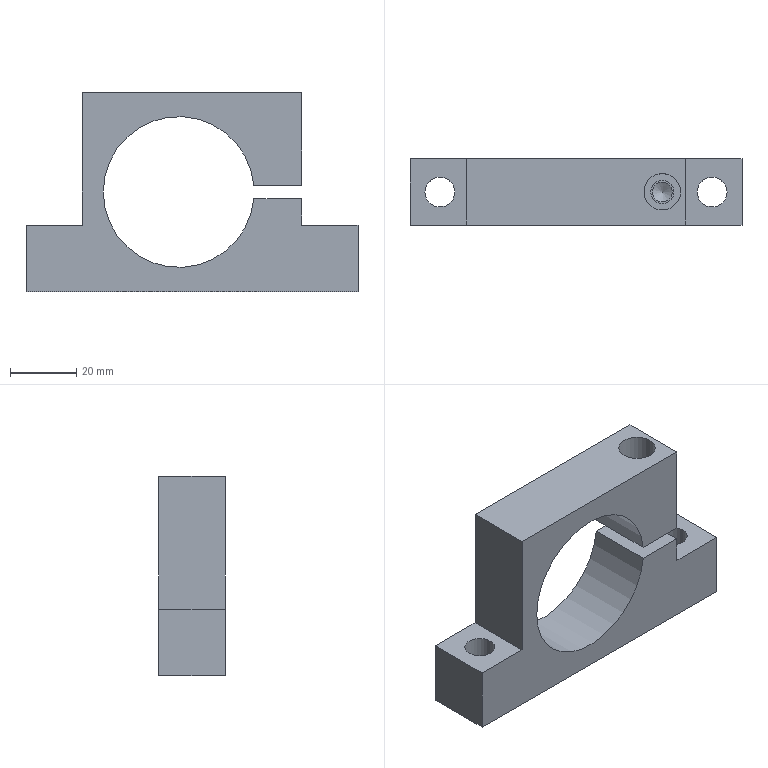Part | NX | features MAIN_BODY 2 | 1 solid | 21 faces | box 100 x 20 x 60 mm | volume 53801 mm3 | plane 14 | cylinder 6 | cone 1 | commonest cylinder face diameters 9 x2 6 x1 7 x1 11 x1 45.4 x1
STEP:
#1=CARTESIAN_POINT('',(568.,600.,-213.));
#2=VERTEX_POINT('',#1);
#3=CARTESIAN_POINT('',(568.,600.,-185.));
#4=VERTEX_POINT('',#3);
#5=CARTESIAN_POINT('',(568.,600.,-185.));
#6=DIRECTION('',(0.,0.,1.));
#7=VECTOR('',#6,1000.);
#8=LINE('',#5,#7);
#9=EDGE_CURVE('',#2,#4,#8,.T.);
#10=ORIENTED_EDGE('',*,*,#9,.F.);
#11=CARTESIAN_POINT('',(568.,620.,-213.));
#12=VERTEX_POINT('',#11);
#13=CARTESIAN_POINT('',(568.,600.,-213.));
#14=DIRECTION('',(0.,-1.,0.));
#15=VECTOR('',#14,1000.);
#16=LINE('',#13,#15);
#17=EDGE_CURVE('',#12,#2,#16,.T.);
#18=ORIENTED_EDGE('',*,*,#17,.F.);
#19=CARTESIAN_POINT('',(568.,620.,-185.));
#20=VERTEX_POINT('',#19);
#21=CARTESIAN_POINT('',(568.,620.,-185.));
#22=DIRECTION('',(0.,0.,1.));
#23=VECTOR('',#22,1000.);
#24=LINE('',#21,#23);
#25=EDGE_CURVE('',#12,#20,#24,.T.);
#26=ORIENTED_EDGE('',*,*,#25,.T.);
#27=CARTESIAN_POINT('',(568.,565.,-185.));
#28=DIRECTION('',(0.,1.,0.));
#29=VECTOR('',#28,1000.);
#30=LINE('',#27,#29);
#31=EDGE_CURVE('',#4,#20,#30,.T.);
#32=ORIENTED_EDGE('',*,*,#31,.F.);
#33=EDGE_LOOP('',(#10,#18,#26,#32));
#34=FACE_BOUND('',#33,.T.);
#35=CARTESIAN_POINT('',(568.,565.,-225.));
#36=DIRECTION('',(-1.,0.,0.));
#37=DIRECTION('',(0.,0.,-1.));
#38=AXIS2_PLACEMENT_3D('',#35,#36,#37);
#39=PLANE('',#38);
#40=ADVANCED_FACE('',(#34),#39,.F.);
#41=CARTESIAN_POINT('',(485.,600.,-225.));
#42=VERTEX_POINT('',#41);
#43=CARTESIAN_POINT('',(485.,620.,-225.));
#44=VERTEX_POINT('',#43);
#45=CARTESIAN_POINT('',(485.,565.,-225.));
#46=DIRECTION('',(0.,1.,0.));
#47=VECTOR('',#46,1000.);
#48=LINE('',#45,#47);
#49=EDGE_CURVE('',#42,#44,#48,.T.);
#50=ORIENTED_EDGE('',*,*,#49,.T.);
#51=CARTESIAN_POINT('',(485.,620.,-245.));
#52=VERTEX_POINT('',#51);
#53=CARTESIAN_POINT('',(485.,620.,-245.));
#54=DIRECTION('',(0.,0.,1.));
#55=VECTOR('',#54,1000.);
#56=LINE('',#53,#55);
#57=EDGE_CURVE('',#52,#44,#56,.T.);
#58=ORIENTED_EDGE('',*,*,#57,.F.);
#59=CARTESIAN_POINT('',(485.,600.,-245.));
#60=VERTEX_POINT('',#59);
#61=CARTESIAN_POINT('',(485.,600.,-245.));
#62=DIRECTION('',(0.,1.,0.));
#63=VECTOR('',#62,1000.);
#64=LINE('',#61,#63);
#65=EDGE_CURVE('',#60,#52,#64,.T.);
#66=ORIENTED_EDGE('',*,*,#65,.F.);
#67=CARTESIAN_POINT('',(485.,600.,-245.));
#68=DIRECTION('',(0.,0.,1.));
#69=VECTOR('',#68,1000.);
#70=LINE('',#67,#69);
#71=EDGE_CURVE('',#60,#42,#70,.T.);
#72=ORIENTED_EDGE('',*,*,#71,.T.);
#73=EDGE_LOOP('',(#50,#58,#66,#72));
#74=FACE_BOUND('',#73,.T.);
#75=CARTESIAN_POINT('',(485.,600.,-245.));
#76=DIRECTION('',(-1.,0.,0.));
#77=DIRECTION('',(0.,0.,-1.));
#78=AXIS2_PLACEMENT_3D('',#75,#76,#77);
#79=PLANE('',#78);
#80=ADVANCED_FACE('',(#74),#79,.T.);
#81=CARTESIAN_POINT('',(555.5,610.,-185.));
#82=VERTEX_POINT('',#81);
#83=CARTESIAN_POINT('',(561.,610.,-185.));
#84=DIRECTION('',(0.,0.,-1.));
#85=DIRECTION('',(-1.,0.,0.));
#86=AXIS2_PLACEMENT_3D('',#83,#84,#85);
#87=CIRCLE('',#86,5.5);
#88=EDGE_CURVE('',#82,#82,#87,.T.);
#89=ORIENTED_EDGE('',*,*,#88,.T.);
#90=EDGE_LOOP('',(#89));
#91=FACE_BOUND('',#90,.T.);
#92=ORIENTED_EDGE('',*,*,#31,.T.);
#93=CARTESIAN_POINT('',(502.,620.,-185.));
#94=VERTEX_POINT('',#93);
#95=CARTESIAN_POINT('',(485.,620.,-185.));
#96=DIRECTION('',(1.,0.,0.));
#97=VECTOR('',#96,1000.);
#98=LINE('',#95,#97);
#99=EDGE_CURVE('',#94,#20,#98,.T.);
#100=ORIENTED_EDGE('',*,*,#99,.F.);
#101=CARTESIAN_POINT('',(502.,600.,-185.));
#102=VERTEX_POINT('',#101);
#103=CARTESIAN_POINT('',(502.,565.,-185.));
#104=DIRECTION('',(0.,1.,0.));
#105=VECTOR('',#104,1000.);
#106=LINE('',#103,#105);
#107=EDGE_CURVE('',#102,#94,#106,.T.);
#108=ORIENTED_EDGE('',*,*,#107,.F.);
#109=CARTESIAN_POINT('',(485.,600.,-185.));
#110=DIRECTION('',(1.,0.,0.));
#111=VECTOR('',#110,1000.);
#112=LINE('',#109,#111);
#113=EDGE_CURVE('',#102,#4,#112,.T.);
#114=ORIENTED_EDGE('',*,*,#113,.T.);
#115=EDGE_LOOP('',(#92,#100,#108,#114));
#116=FACE_BOUND('',#115,.T.);
#117=CARTESIAN_POINT('',(485.,600.,-185.));
#118=DIRECTION('',(0.,0.,1.));
#119=DIRECTION('',(0.,-1.,0.));
#120=AXIS2_PLACEMENT_3D('',#117,#118,#119);
#121=PLANE('',#120);
#122=ADVANCED_FACE('',(#91,#116),#121,.T.);
#123=CARTESIAN_POINT('',(585.,600.,-225.));
#124=VERTEX_POINT('',#123);
#125=CARTESIAN_POINT('',(585.,620.,-225.));
#126=VERTEX_POINT('',#125);
#127=CARTESIAN_POINT('',(585.,565.,-225.));
#128=DIRECTION('',(0.,1.,0.));
#129=VECTOR('',#128,1000.);
#130=LINE('',#127,#129);
#131=EDGE_CURVE('',#124,#126,#130,.T.);
#132=ORIENTED_EDGE('',*,*,#131,.F.);
#133=CARTESIAN_POINT('',(585.,600.,-245.));
#134=VERTEX_POINT('',#133);
#135=CARTESIAN_POINT('',(585.,600.,-185.));
#136=DIRECTION('',(0.,0.,-1.));
#137=VECTOR('',#136,1000.);
#138=LINE('',#135,#137);
#139=EDGE_CURVE('',#124,#134,#138,.T.);
#140=ORIENTED_EDGE('',*,*,#139,.T.);
#141=CARTESIAN_POINT('',(585.,620.,-245.));
#142=VERTEX_POINT('',#141);
#143=CARTESIAN_POINT('',(585.,600.,-245.));
#144=DIRECTION('',(0.,1.,0.));
#145=VECTOR('',#144,1000.);
#146=LINE('',#143,#145);
#147=EDGE_CURVE('',#134,#142,#146,.T.);
#148=ORIENTED_EDGE('',*,*,#147,.T.);
#149=CARTESIAN_POINT('',(585.,620.,-185.));
#150=DIRECTION('',(0.,0.,-1.));
#151=VECTOR('',#150,1000.);
#152=LINE('',#149,#151);
#153=EDGE_CURVE('',#126,#142,#152,.T.);
#154=ORIENTED_EDGE('',*,*,#153,.F.);
#155=EDGE_LOOP('',(#132,#140,#148,#154));
#156=FACE_BOUND('',#155,.T.);
#157=CARTESIAN_POINT('',(585.,600.,-185.));
#158=DIRECTION('',(1.,0.,0.));
#159=DIRECTION('',(0.,0.,1.));
#160=AXIS2_PLACEMENT_3D('',#157,#158,#159);
#161=PLANE('',#160);
#162=ADVANCED_FACE('',(#156),#161,.T.);
#163=CARTESIAN_POINT('',(580.5,610.,-245.));
#164=VERTEX_POINT('',#163);
#165=CARTESIAN_POINT('',(576.,610.,-245.));
#166=DIRECTION('',(0.,0.,-1.));
#167=DIRECTION('',(1.,0.,0.));
#168=AXIS2_PLACEMENT_3D('',#165,#166,#167);
#169=CIRCLE('',#168,4.5);
#170=EDGE_CURVE('',#164,#164,#169,.T.);
#171=ORIENTED_EDGE('',*,*,#170,.F.);
#172=EDGE_LOOP('',(#171));
#173=FACE_BOUND('',#172,.T.);
#174=CARTESIAN_POINT('',(498.5,610.,-245.));
#175=VERTEX_POINT('',#174);
#176=CARTESIAN_POINT('',(494.,610.,-245.));
#177=DIRECTION('',(0.,0.,-1.));
#178=DIRECTION('',(1.,0.,0.));
#179=AXIS2_PLACEMENT_3D('',#176,#177,#178);
#180=CIRCLE('',#179,4.5);
#181=EDGE_CURVE('',#175,#175,#180,.T.);
#182=ORIENTED_EDGE('',*,*,#181,.F.);
#183=EDGE_LOOP('',(#182));
#184=FACE_BOUND('',#183,.T.);
#185=CARTESIAN_POINT('',(585.,620.,-245.));
#186=DIRECTION('',(-1.,0.,0.));
#187=VECTOR('',#186,1000.);
#188=LINE('',#185,#187);
#189=EDGE_CURVE('',#142,#52,#188,.T.);
#190=ORIENTED_EDGE('',*,*,#189,.F.);
#191=ORIENTED_EDGE('',*,*,#147,.F.);
#192=CARTESIAN_POINT('',(585.,600.,-245.));
#193=DIRECTION('',(-1.,0.,0.));
#194=VECTOR('',#193,1000.);
#195=LINE('',#192,#194);
#196=EDGE_CURVE('',#134,#60,#195,.T.);
#197=ORIENTED_EDGE('',*,*,#196,.T.);
#198=ORIENTED_EDGE('',*,*,#65,.T.);
#199=EDGE_LOOP('',(#190,#191,#197,#198));
#200=FACE_BOUND('',#199,.T.);
#201=CARTESIAN_POINT('',(585.,600.,-245.));
#202=DIRECTION('',(0.,0.,-1.));
#203=DIRECTION('',(1.,0.,0.));
#204=AXIS2_PLACEMENT_3D('',#201,#202,#203);
#205=PLANE('',#204);
#206=ADVANCED_FACE('',(#173,#184,#200),#205,.T.);
#207=CARTESIAN_POINT('',(553.612,600.,-213.));
#208=VERTEX_POINT('',#207);
#209=CARTESIAN_POINT('',(553.612,620.,-213.));
#210=VERTEX_POINT('',#209);
#211=CARTESIAN_POINT('',(553.612,600.,-213.));
#212=DIRECTION('',(0.,1.,0.));
#213=VECTOR('',#212,1000.);
#214=LINE('',#211,#213);
#215=EDGE_CURVE('',#208,#210,#214,.T.);
#216=ORIENTED_EDGE('',*,*,#215,.F.);
#217=CARTESIAN_POINT('',(553.612,600.,-217.));
#218=VERTEX_POINT('',#217);
#219=CARTESIAN_POINT('',(531.,600.,-215.));
#220=DIRECTION('',(0.,-1.,0.));
#221=DIRECTION('',(1.,0.,0.));
#222=AXIS2_PLACEMENT_3D('',#219,#220,#221);
#223=CIRCLE('',#222,22.7);
#224=EDGE_CURVE('',#208,#218,#223,.T.);
#225=ORIENTED_EDGE('',*,*,#224,.T.);
#226=CARTESIAN_POINT('',(553.612,620.,-217.));
#227=VERTEX_POINT('',#226);
#228=CARTESIAN_POINT('',(553.612,600.,-217.));
#229=DIRECTION('',(0.,1.,0.));
#230=VECTOR('',#229,1000.);
#231=LINE('',#228,#230);
#232=EDGE_CURVE('',#227,#218,#231,.F.);
#233=ORIENTED_EDGE('',*,*,#232,.F.);
#234=CARTESIAN_POINT('',(531.,620.,-215.));
#235=DIRECTION('',(0.,-1.,0.));
#236=DIRECTION('',(1.,0.,0.));
#237=AXIS2_PLACEMENT_3D('',#234,#235,#236);
#238=CIRCLE('',#237,22.7);
#239=EDGE_CURVE('',#210,#227,#238,.T.);
#240=ORIENTED_EDGE('',*,*,#239,.F.);
#241=EDGE_LOOP('',(#216,#225,#233,#240));
#242=FACE_BOUND('',#241,.T.);
#243=CARTESIAN_POINT('',(531.,600.,-215.));
#244=DIRECTION('',(0.,1.,0.));
#245=DIRECTION('',(-1.,0.,0.));
#246=AXIS2_PLACEMENT_3D('',#243,#244,#245);
#247=CYLINDRICAL_SURFACE('',#246,22.7);
#248=ADVANCED_FACE('',(#242),#247,.F.);
#249=ORIENTED_EDGE('',*,*,#224,.F.);
#250=CARTESIAN_POINT('',(531.,600.,-213.));
#251=DIRECTION('',(1.,0.,0.));
#252=VECTOR('',#251,1000.);
#253=LINE('',#250,#252);
#254=EDGE_CURVE('',#208,#2,#253,.T.);
#255=ORIENTED_EDGE('',*,*,#254,.T.);
#256=ORIENTED_EDGE('',*,*,#9,.T.);
#257=ORIENTED_EDGE('',*,*,#113,.F.);
#258=CARTESIAN_POINT('',(502.,600.,-225.));
#259=VERTEX_POINT('',#258);
#260=CARTESIAN_POINT('',(502.,600.,-185.));
#261=DIRECTION('',(0.,0.,-1.));
#262=VECTOR('',#261,1000.);
#263=LINE('',#260,#262);
#264=EDGE_CURVE('',#102,#259,#263,.T.);
#265=ORIENTED_EDGE('',*,*,#264,.T.);
#266=CARTESIAN_POINT('',(485.,600.,-225.));
#267=DIRECTION('',(-1.,0.,0.));
#268=VECTOR('',#267,1000.);
#269=LINE('',#266,#268);
#270=EDGE_CURVE('',#259,#42,#269,.T.);
#271=ORIENTED_EDGE('',*,*,#270,.T.);
#272=ORIENTED_EDGE('',*,*,#71,.F.);
#273=ORIENTED_EDGE('',*,*,#196,.F.);
#274=ORIENTED_EDGE('',*,*,#139,.F.);
#275=CARTESIAN_POINT('',(568.,600.,-225.));
#276=VERTEX_POINT('',#275);
#277=CARTESIAN_POINT('',(485.,600.,-225.));
#278=DIRECTION('',(-1.,0.,0.));
#279=VECTOR('',#278,1000.);
#280=LINE('',#277,#279);
#281=EDGE_CURVE('',#124,#276,#280,.T.);
#282=ORIENTED_EDGE('',*,*,#281,.T.);
#283=CARTESIAN_POINT('',(568.,600.,-217.));
#284=VERTEX_POINT('',#283);
#285=CARTESIAN_POINT('',(568.,600.,-185.));
#286=DIRECTION('',(0.,0.,1.));
#287=VECTOR('',#286,1000.);
#288=LINE('',#285,#287);
#289=EDGE_CURVE('',#276,#284,#288,.T.);
#290=ORIENTED_EDGE('',*,*,#289,.T.);
#291=CARTESIAN_POINT('',(531.,600.,-217.));
#292=DIRECTION('',(1.,0.,0.));
#293=VECTOR('',#292,1000.);
#294=LINE('',#291,#293);
#295=EDGE_CURVE('',#218,#284,#294,.T.);
#296=ORIENTED_EDGE('',*,*,#295,.F.);
#297=EDGE_LOOP('',(#249,#255,#256,#257,#265,#271,#272,#273,#274,#282,#290,#296));
#298=FACE_BOUND('',#297,.T.);
#299=CARTESIAN_POINT('',(485.,600.,-185.));
#300=DIRECTION('',(0.,1.,0.));
#301=DIRECTION('',(-1.,0.,0.));
#302=AXIS2_PLACEMENT_3D('',#299,#300,#301);
#303=PLANE('',#302);
#304=ADVANCED_FACE('',(#298),#303,.F.);
#305=CARTESIAN_POINT('',(485.,620.,-213.));
#306=DIRECTION('',(1.,0.,0.));
#307=VECTOR('',#306,1000.);
#308=LINE('',#305,#307);
#309=EDGE_CURVE('',#210,#12,#308,.T.);
#310=ORIENTED_EDGE('',*,*,#309,.F.);
#311=ORIENTED_EDGE('',*,*,#239,.T.);
#312=CARTESIAN_POINT('',(568.,620.,-217.));
#313=VERTEX_POINT('',#312);
#314=CARTESIAN_POINT('',(485.,620.,-217.));
#315=DIRECTION('',(1.,0.,0.));
#316=VECTOR('',#315,1000.);
#317=LINE('',#314,#316);
#318=EDGE_CURVE('',#313,#227,#317,.F.);
#319=ORIENTED_EDGE('',*,*,#318,.F.);
#320=CARTESIAN_POINT('',(568.,620.,-225.));
#321=VERTEX_POINT('',#320);
#322=CARTESIAN_POINT('',(568.,620.,-185.));
#323=DIRECTION('',(0.,0.,1.));
#324=VECTOR('',#323,1000.);
#325=LINE('',#322,#324);
#326=EDGE_CURVE('',#321,#313,#325,.T.);
#327=ORIENTED_EDGE('',*,*,#326,.F.);
#328=CARTESIAN_POINT('',(485.,620.,-225.));
#329=DIRECTION('',(-1.,0.,0.));
#330=VECTOR('',#329,1000.);
#331=LINE('',#328,#330);
#332=EDGE_CURVE('',#126,#321,#331,.T.);
#333=ORIENTED_EDGE('',*,*,#332,.F.);
#334=ORIENTED_EDGE('',*,*,#153,.T.);
#335=ORIENTED_EDGE('',*,*,#189,.T.);
#336=ORIENTED_EDGE('',*,*,#57,.T.);
#337=CARTESIAN_POINT('',(502.,620.,-225.));
#338=VERTEX_POINT('',#337);
#339=CARTESIAN_POINT('',(485.,620.,-225.));
#340=DIRECTION('',(-1.,0.,0.));
#341=VECTOR('',#340,1000.);
#342=LINE('',#339,#341);
#343=EDGE_CURVE('',#338,#44,#342,.T.);
#344=ORIENTED_EDGE('',*,*,#343,.F.);
#345=CARTESIAN_POINT('',(502.,620.,-185.));
#346=DIRECTION('',(0.,0.,-1.));
#347=VECTOR('',#346,1000.);
#348=LINE('',#345,#347);
#349=EDGE_CURVE('',#94,#338,#348,.T.);
#350=ORIENTED_EDGE('',*,*,#349,.F.);
#351=ORIENTED_EDGE('',*,*,#99,.T.);
#352=ORIENTED_EDGE('',*,*,#25,.F.);
#353=EDGE_LOOP('',(#310,#311,#319,#327,#333,#334,#335,#336,#344,#350,#351,#352));
#354=FACE_BOUND('',#353,.T.);
#355=CARTESIAN_POINT('',(485.,620.,-185.));
#356=DIRECTION('',(0.,1.,0.));
#357=DIRECTION('',(-1.,0.,0.));
#358=AXIS2_PLACEMENT_3D('',#355,#356,#357);
#359=PLANE('',#358);
#360=ADVANCED_FACE('',(#354),#359,.T.);
#361=ORIENTED_EDGE('',*,*,#107,.T.);
#362=ORIENTED_EDGE('',*,*,#349,.T.);
#363=CARTESIAN_POINT('',(502.,565.,-225.));
#364=DIRECTION('',(0.,1.,0.));
#365=VECTOR('',#364,1000.);
#366=LINE('',#363,#365);
#367=EDGE_CURVE('',#259,#338,#366,.T.);
#368=ORIENTED_EDGE('',*,*,#367,.F.);
#369=ORIENTED_EDGE('',*,*,#264,.F.);
#370=EDGE_LOOP('',(#361,#362,#368,#369));
#371=FACE_BOUND('',#370,.T.);
#372=CARTESIAN_POINT('',(502.,565.,-185.));
#373=DIRECTION('',(1.,0.,0.));
#374=DIRECTION('',(0.,0.,1.));
#375=AXIS2_PLACEMENT_3D('',#372,#373,#374);
#376=PLANE('',#375);
#377=ADVANCED_FACE('',(#371),#376,.F.);
#378=CARTESIAN_POINT('',(498.5,610.,-225.));
#379=VERTEX_POINT('',#378);
#380=CARTESIAN_POINT('',(494.,610.,-225.));
#381=DIRECTION('',(0.,0.,-1.));
#382=DIRECTION('',(1.,0.,0.));
#383=AXIS2_PLACEMENT_3D('',#380,#381,#382);
#384=CIRCLE('',#383,4.5);
#385=EDGE_CURVE('',#379,#379,#384,.T.);
#386=ORIENTED_EDGE('',*,*,#385,.T.);
#387=EDGE_LOOP('',(#386));
#388=FACE_BOUND('',#387,.T.);
#389=ORIENTED_EDGE('',*,*,#367,.T.);
#390=ORIENTED_EDGE('',*,*,#343,.T.);
#391=ORIENTED_EDGE('',*,*,#49,.F.);
#392=ORIENTED_EDGE('',*,*,#270,.F.);
#393=EDGE_LOOP('',(#389,#390,#391,#392));
#394=FACE_BOUND('',#393,.T.);
#395=CARTESIAN_POINT('',(502.,565.,-225.));
#396=DIRECTION('',(0.,0.,-1.));
#397=DIRECTION('',(1.,0.,0.));
#398=AXIS2_PLACEMENT_3D('',#395,#396,#397);
#399=PLANE('',#398);
#400=ADVANCED_FACE('',(#388,#394),#399,.F.);
#401=CARTESIAN_POINT('',(580.5,610.,-225.));
#402=VERTEX_POINT('',#401);
#403=CARTESIAN_POINT('',(576.,610.,-225.));
#404=DIRECTION('',(0.,0.,-1.));
#405=DIRECTION('',(1.,0.,0.));
#406=AXIS2_PLACEMENT_3D('',#403,#404,#405);
#407=CIRCLE('',#406,4.5);
#408=EDGE_CURVE('',#402,#402,#407,.T.);
#409=ORIENTED_EDGE('',*,*,#408,.T.);
#410=EDGE_LOOP('',(#409));
#411=FACE_BOUND('',#410,.T.);
#412=ORIENTED_EDGE('',*,*,#131,.T.);
#413=ORIENTED_EDGE('',*,*,#332,.T.);
#414=CARTESIAN_POINT('',(568.,565.,-225.));
#415=DIRECTION('',(0.,1.,0.));
#416=VECTOR('',#415,1000.);
#417=LINE('',#414,#416);
#418=EDGE_CURVE('',#276,#321,#417,.T.);
#419=ORIENTED_EDGE('',*,*,#418,.F.);
#420=ORIENTED_EDGE('',*,*,#281,.F.);
#421=EDGE_LOOP('',(#412,#413,#419,#420));
#422=FACE_BOUND('',#421,.T.);
#423=CARTESIAN_POINT('',(585.,565.,-225.));
#424=DIRECTION('',(0.,0.,-1.));
#425=DIRECTION('',(1.,0.,0.));
#426=AXIS2_PLACEMENT_3D('',#423,#424,#425);
#427=PLANE('',#426);
#428=ADVANCED_FACE('',(#411,#422),#427,.F.);
#429=ORIENTED_EDGE('',*,*,#326,.T.);
#430=CARTESIAN_POINT('',(568.,600.,-217.));
#431=DIRECTION('',(0.,-1.,0.));
#432=VECTOR('',#431,1000.);
#433=LINE('',#430,#432);
#434=EDGE_CURVE('',#313,#284,#433,.T.);
#435=ORIENTED_EDGE('',*,*,#434,.T.);
#436=ORIENTED_EDGE('',*,*,#289,.F.);
#437=ORIENTED_EDGE('',*,*,#418,.T.);
#438=EDGE_LOOP('',(#429,#435,#436,#437));
#439=FACE_BOUND('',#438,.T.);
#440=CARTESIAN_POINT('',(568.,565.,-225.));
#441=DIRECTION('',(-1.,0.,0.));
#442=DIRECTION('',(0.,0.,-1.));
#443=AXIS2_PLACEMENT_3D('',#440,#441,#442);
#444=PLANE('',#443);
#445=ADVANCED_FACE('',(#439),#444,.F.);
#446=ORIENTED_EDGE('',*,*,#181,.T.);
#447=EDGE_LOOP('',(#446));
#448=FACE_BOUND('',#447,.T.);
#449=ORIENTED_EDGE('',*,*,#385,.F.);
#450=EDGE_LOOP('',(#449));
#451=FACE_BOUND('',#450,.T.);
#452=CARTESIAN_POINT('',(494.,610.,-255.));
#453=DIRECTION('',(0.,0.,1.));
#454=DIRECTION('',(0.,-1.,0.));
#455=AXIS2_PLACEMENT_3D('',#452,#453,#454);
#456=CYLINDRICAL_SURFACE('',#455,4.5);
#457=ADVANCED_FACE('',(#448,#451),#456,.F.);
#458=ORIENTED_EDGE('',*,*,#170,.T.);
#459=EDGE_LOOP('',(#458));
#460=FACE_BOUND('',#459,.T.);
#461=ORIENTED_EDGE('',*,*,#408,.F.);
#462=EDGE_LOOP('',(#461));
#463=FACE_BOUND('',#462,.T.);
#464=CARTESIAN_POINT('',(576.,610.,-255.));
#465=DIRECTION('',(0.,0.,1.));
#466=DIRECTION('',(0.,-1.,0.));
#467=AXIS2_PLACEMENT_3D('',#464,#465,#466);
#468=CYLINDRICAL_SURFACE('',#467,4.5);
#469=ADVANCED_FACE('',(#460,#463),#468,.F.);
#470=CARTESIAN_POINT('',(558.,610.,-217.));
#471=VERTEX_POINT('',#470);
#472=CARTESIAN_POINT('',(561.,610.,-217.));
#473=DIRECTION('',(0.,0.,-1.));
#474=DIRECTION('',(-1.,0.,0.));
#475=AXIS2_PLACEMENT_3D('',#472,#473,#474);
#476=CIRCLE('',#475,3.);
#477=EDGE_CURVE('',#471,#471,#476,.T.);
#478=ORIENTED_EDGE('',*,*,#477,.T.);
#479=EDGE_LOOP('',(#478));
#480=FACE_BOUND('',#479,.T.);
#481=ORIENTED_EDGE('',*,*,#232,.T.);
#482=ORIENTED_EDGE('',*,*,#295,.T.);
#483=ORIENTED_EDGE('',*,*,#434,.F.);
#484=ORIENTED_EDGE('',*,*,#318,.T.);
#485=EDGE_LOOP('',(#481,#482,#483,#484));
#486=FACE_BOUND('',#485,.T.);
#487=CARTESIAN_POINT('',(531.,600.,-217.));
#488=DIRECTION('',(0.,0.,1.));
#489=DIRECTION('',(1.,0.,0.));
#490=AXIS2_PLACEMENT_3D('',#487,#488,#489);
#491=PLANE('',#490);
#492=ADVANCED_FACE('',(#480,#486),#491,.T.);
#493=CARTESIAN_POINT('',(564.5,610.,-213.));
#494=VERTEX_POINT('',#493);
#495=CARTESIAN_POINT('',(561.,610.,-213.));
#496=DIRECTION('',(0.,0.,1.));
#497=DIRECTION('',(1.,0.,0.));
#498=AXIS2_PLACEMENT_3D('',#495,#496,#497);
#499=CIRCLE('',#498,3.5);
#500=EDGE_CURVE('',#494,#494,#499,.T.);
#501=ORIENTED_EDGE('',*,*,#500,.T.);
#502=EDGE_LOOP('',(#501));
#503=FACE_BOUND('',#502,.T.);
#504=ORIENTED_EDGE('',*,*,#215,.T.);
#505=ORIENTED_EDGE('',*,*,#309,.T.);
#506=ORIENTED_EDGE('',*,*,#17,.T.);
#507=ORIENTED_EDGE('',*,*,#254,.F.);
#508=EDGE_LOOP('',(#504,#505,#506,#507));
#509=FACE_BOUND('',#508,.T.);
#510=CARTESIAN_POINT('',(531.,600.,-213.));
#511=DIRECTION('',(0.,0.,1.));
#512=DIRECTION('',(1.,0.,0.));
#513=AXIS2_PLACEMENT_3D('',#510,#511,#512);
#514=PLANE('',#513);
#515=ADVANCED_FACE('',(#503,#509),#514,.F.);
#516=CARTESIAN_POINT('',(557.5,610.,-205.));
#517=VERTEX_POINT('',#516);
#518=CARTESIAN_POINT('',(561.,610.,-205.));
#519=DIRECTION('',(0.,0.,-1.));
#520=DIRECTION('',(-1.,0.,0.));
#521=AXIS2_PLACEMENT_3D('',#518,#519,#520);
#522=CIRCLE('',#521,3.5);
#523=EDGE_CURVE('',#517,#517,#522,.T.);
#524=ORIENTED_EDGE('',*,*,#523,.F.);
#525=EDGE_LOOP('',(#524));
#526=FACE_BOUND('',#525,.T.);
#527=ORIENTED_EDGE('',*,*,#500,.F.);
#528=EDGE_LOOP('',(#527));
#529=FACE_BOUND('',#528,.T.);
#530=CARTESIAN_POINT('',(561.,610.,-215.));
#531=DIRECTION('',(0.,0.,-1.));
#532=DIRECTION('',(-1.,0.,0.));
#533=AXIS2_PLACEMENT_3D('',#530,#531,#532);
#534=CYLINDRICAL_SURFACE('',#533,3.5);
#535=ADVANCED_FACE('',(#526,#529),#534,.F.);
#536=ORIENTED_EDGE('',*,*,#523,.T.);
#537=EDGE_LOOP('',(#536));
#538=FACE_BOUND('',#537,.T.);
#539=CARTESIAN_POINT('',(555.5,610.,-205.));
#540=VERTEX_POINT('',#539);
#541=CARTESIAN_POINT('',(561.,610.,-205.));
#542=DIRECTION('',(0.,0.,-1.));
#543=DIRECTION('',(-1.,0.,0.));
#544=AXIS2_PLACEMENT_3D('',#541,#542,#543);
#545=CIRCLE('',#544,5.5);
#546=EDGE_CURVE('',#540,#540,#545,.T.);
#547=ORIENTED_EDGE('',*,*,#546,.F.);
#548=EDGE_LOOP('',(#547));
#549=FACE_BOUND('',#548,.T.);
#550=CARTESIAN_POINT('',(561.,610.,-205.));
#551=DIRECTION('',(0.,0.,-1.));
#552=DIRECTION('',(-1.,0.,0.));
#553=AXIS2_PLACEMENT_3D('',#550,#551,#552);
#554=PLANE('',#553);
#555=ADVANCED_FACE('',(#538,#549),#554,.F.);
#556=ORIENTED_EDGE('',*,*,#546,.T.);
#557=EDGE_LOOP('',(#556));
#558=FACE_BOUND('',#557,.T.);
#559=ORIENTED_EDGE('',*,*,#88,.F.);
#560=EDGE_LOOP('',(#559));
#561=FACE_BOUND('',#560,.T.);
#562=CARTESIAN_POINT('',(561.,610.,-185.));
#563=DIRECTION('',(0.,0.,-1.));
#564=DIRECTION('',(-1.,0.,0.));
#565=AXIS2_PLACEMENT_3D('',#562,#563,#564);
#566=CYLINDRICAL_SURFACE('',#565,5.5);
#567=ADVANCED_FACE('',(#558,#561),#566,.F.);
#568=CARTESIAN_POINT('',(558.,610.,-242.));
#569=VERTEX_POINT('',#568);
#570=CARTESIAN_POINT('',(561.,610.,-242.));
#571=DIRECTION('',(0.,0.,-1.));
#572=DIRECTION('',(-1.,0.,0.));
#573=AXIS2_PLACEMENT_3D('',#570,#571,#572);
#574=CIRCLE('',#573,3.);
#575=EDGE_CURVE('',#569,#569,#574,.T.);
#576=ORIENTED_EDGE('',*,*,#575,.F.);
#577=EDGE_LOOP('',(#576));
#578=FACE_BOUND('',#577,.T.);
#579=CARTESIAN_POINT('',(561.,610.,-243.732));
#580=VERTEX_POINT('',#579);
#581=VERTEX_LOOP('',#580);
#582=FACE_BOUND('',#581,.T.);
#583=CARTESIAN_POINT('',(561.,610.,-242.));
#584=DIRECTION('',(0.,0.,1.));
#585=DIRECTION('',(1.,0.,0.));
#586=AXIS2_PLACEMENT_3D('',#583,#584,#585);
#587=CONICAL_SURFACE('',#586,3.,1.047);
#588=ADVANCED_FACE('',(#578,#582),#587,.F.);
#589=ORIENTED_EDGE('',*,*,#575,.T.);
#590=EDGE_LOOP('',(#589));
#591=FACE_BOUND('',#590,.T.);
#592=ORIENTED_EDGE('',*,*,#477,.F.);
#593=EDGE_LOOP('',(#592));
#594=FACE_BOUND('',#593,.T.);
#595=CARTESIAN_POINT('',(561.,610.,-217.));
#596=DIRECTION('',(0.,0.,-1.));
#597=DIRECTION('',(-1.,0.,0.));
#598=AXIS2_PLACEMENT_3D('',#595,#596,#597);
#599=CYLINDRICAL_SURFACE('',#598,3.);
#600=ADVANCED_FACE('',(#591,#594),#599,.F.);
#601=CLOSED_SHELL('',(#40,#80,#122,#162,#206,#248,#304,#360,#377,#400,#428,#445,#457,#469,#492,#515,#535,#555,#567,#588,#600));
#602=MANIFOLD_SOLID_BREP('',#601);
#603=(LENGTH_UNIT()NAMED_UNIT(*)SI_UNIT(.MILLI.,.METRE.));
#604=UNCERTAINTY_MEASURE_WITH_UNIT(LENGTH_MEASURE(0.00001),#603,'','');
#605=(NAMED_UNIT(*)PLANE_ANGLE_UNIT()SI_UNIT($,.RADIAN.));
#606=(NAMED_UNIT(*)SI_UNIT($,.STERADIAN.)SOLID_ANGLE_UNIT());
#607=(GEOMETRIC_REPRESENTATION_CONTEXT(3)GLOBAL_UNCERTAINTY_ASSIGNED_CONTEXT((#604))GLOBAL_UNIT_ASSIGNED_CONTEXT((#603,#605,#606))REPRESENTATION_CONTEXT('',''));
#608=ADVANCED_BREP_SHAPE_REPRESENTATION('',(#602),#607);